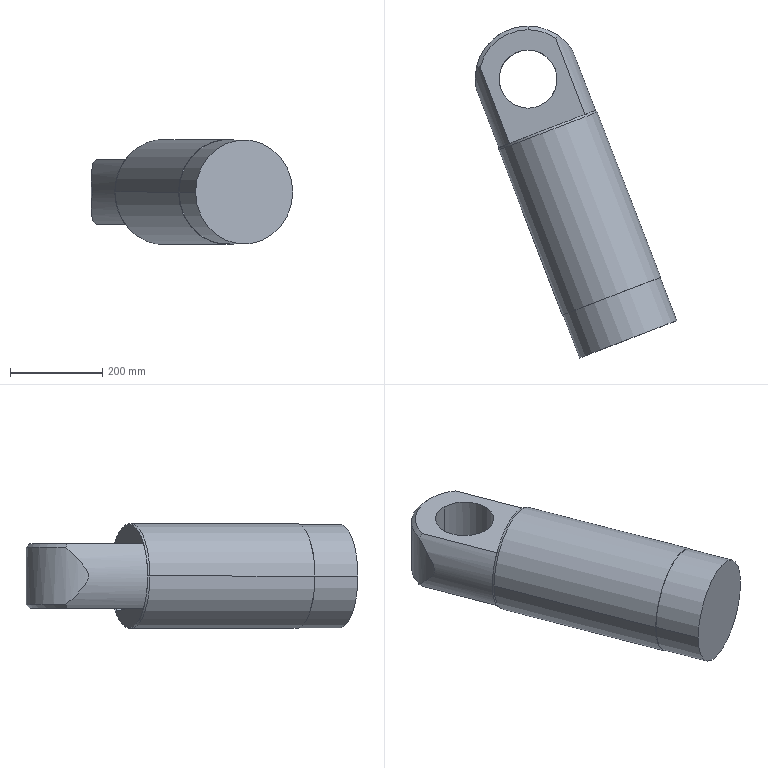Part | SolidWorks | features MoveFace 2, BaseBody 1, Scale 1 | 1 solid | 20 faces | box 436.641 x 719.533 x 228 mm | volume 24273606 mm3 | cylinder 10 | cone 5 | plane 5 | commonest cylinder face diameters 224.4 x3 228 x3 126 x2 225.6 x2
STEP:
#1=CARTESIAN_POINT('',(450.61,-136.711,89.501));
#2=VERTEX_POINT('',#1);
#3=CARTESIAN_POINT('',(237.813,-218.572,89.501));
#4=VERTEX_POINT('',#3);
#5=CARTESIAN_POINT('',(344.212,-177.641,89.501));
#6=DIRECTION('',(0.359,-0.9333,-0.000000526));
#7=DIRECTION('',(0.9333,0.359,0.));
#8=AXIS2_PLACEMENT_3D('',#5,#6,#7);
#9=CIRCLE('',#8,114.);
#10=EDGE_CURVE('',#2,#4,#9,.T.);
#11=ORIENTED_EDGE('',*,*,#10,.T.);
#12=CARTESIAN_POINT('',(375.469,-576.408,89.5));
#13=VERTEX_POINT('',#12);
#14=CARTESIAN_POINT('',(236.09,-214.092,89.501));
#15=DIRECTION('',(0.359,-0.9333,-0.000000526));
#16=VECTOR('',#15,1000.);
#17=LINE('',#14,#16);
#18=EDGE_CURVE('',#4,#13,#17,.T.);
#19=ORIENTED_EDGE('',*,*,#18,.T.);
#20=CARTESIAN_POINT('',(588.266,-494.547,89.5));
#21=VERTEX_POINT('',#20);
#22=CARTESIAN_POINT('',(481.867,-535.477,89.5));
#23=DIRECTION('',(-0.359,0.9333,0.000000526));
#24=DIRECTION('',(0.9333,0.359,0.));
#25=AXIS2_PLACEMENT_3D('',#22,#23,#24);
#26=CIRCLE('',#25,114.);
#27=EDGE_CURVE('',#13,#21,#26,.T.);
#28=ORIENTED_EDGE('',*,*,#27,.T.);
#29=CARTESIAN_POINT('',(448.887,-132.231,89.501));
#30=DIRECTION('',(0.359,-0.9333,-0.000000526));
#31=VECTOR('',#30,1000.);
#32=LINE('',#29,#31);
#33=EDGE_CURVE('',#2,#21,#32,.T.);
#34=ORIENTED_EDGE('',*,*,#33,.F.);
#35=EDGE_LOOP('',(#11,#19,#28,#34));
#36=FACE_OUTER_BOUND('',#35,.T.);
#37=CARTESIAN_POINT('',(342.488,-173.161,89.501));
#38=DIRECTION('',(0.359,-0.9333,-0.000000526));
#39=DIRECTION('',(0.9333,0.359,0.));
#40=AXIS2_PLACEMENT_3D('',#37,#38,#39);
#41=CYLINDRICAL_SURFACE('',#40,114.);
#42=ADVANCED_FACE('',(#36),#41,.T.);
#43=CARTESIAN_POINT('',(447.256,-132.858,89.501));
#44=VERTEX_POINT('',#43);
#45=CARTESIAN_POINT('',(237.72,-213.465,89.501));
#46=VERTEX_POINT('',#45);
#47=CARTESIAN_POINT('',(342.488,-173.161,89.501));
#48=DIRECTION('',(0.359,-0.9333,-0.000000526));
#49=DIRECTION('',(0.9333,0.359,0.));
#50=AXIS2_PLACEMENT_3D('',#47,#48,#49);
#51=CIRCLE('',#50,112.253);
#52=EDGE_CURVE('',#44,#46,#51,.T.);
#53=ORIENTED_EDGE('',*,*,#52,.T.);
#54=CARTESIAN_POINT('',(237.813,-218.572,89.501));
#55=DIRECTION('',(0.01817,-0.9998,-0.000000494));
#56=VECTOR('',#55,1000.);
#57=LINE('',#54,#56);
#58=EDGE_CURVE('',#46,#4,#57,.T.);
#59=ORIENTED_EDGE('',*,*,#58,.T.);
#60=ORIENTED_EDGE('',*,*,#10,.F.);
#61=CARTESIAN_POINT('',(450.61,-136.711,89.501));
#62=DIRECTION('',(0.6566,-0.7542,-0.000000494));
#63=VECTOR('',#62,1000.);
#64=LINE('',#61,#63);
#65=EDGE_CURVE('',#44,#2,#64,.T.);
#66=ORIENTED_EDGE('',*,*,#65,.F.);
#67=EDGE_LOOP('',(#53,#59,#60,#66));
#68=FACE_OUTER_BOUND('',#67,.T.);
#69=CARTESIAN_POINT('',(344.212,-177.641,89.501));
#70=DIRECTION('',(0.359,-0.9333,-0.000000526));
#71=DIRECTION('',(0.9333,0.359,0.));
#72=AXIS2_PLACEMENT_3D('',#69,#70,#71);
#73=CONICAL_SURFACE('',#72,114.,0.3491);
#74=ADVANCED_FACE('',(#68),#73,.T.);
#75=CARTESIAN_POINT('',(376.589,-575.977,89.5));
#76=VERTEX_POINT('',#75);
#77=CARTESIAN_POINT('',(587.146,-494.977,89.5));
#78=VERTEX_POINT('',#77);
#79=CARTESIAN_POINT('',(481.867,-535.477,89.5));
#80=DIRECTION('',(-0.359,0.9333,0.000000526));
#81=DIRECTION('',(0.9333,0.359,0.));
#82=AXIS2_PLACEMENT_3D('',#79,#80,#81);
#83=CIRCLE('',#82,112.8);
#84=EDGE_CURVE('',#76,#78,#83,.T.);
#85=ORIENTED_EDGE('',*,*,#84,.F.);
#86=CARTESIAN_POINT('',(412.564,-669.496,89.5));
#87=VERTEX_POINT('',#86);
#88=CARTESIAN_POINT('',(376.589,-575.977,89.5));
#89=DIRECTION('',(0.359,-0.9333,-0.000000526));
#90=VECTOR('',#89,1000.);
#91=LINE('',#88,#90);
#92=EDGE_CURVE('',#76,#87,#91,.T.);
#93=ORIENTED_EDGE('',*,*,#92,.T.);
#94=CARTESIAN_POINT('',(623.122,-588.496,89.5));
#95=VERTEX_POINT('',#94);
#96=CARTESIAN_POINT('',(517.843,-628.996,89.5));
#97=DIRECTION('',(-0.359,0.9333,0.000000526));
#98=DIRECTION('',(0.9333,0.359,0.));
#99=AXIS2_PLACEMENT_3D('',#96,#97,#98);
#100=CIRCLE('',#99,112.8);
#101=EDGE_CURVE('',#87,#95,#100,.T.);
#102=ORIENTED_EDGE('',*,*,#101,.T.);
#103=CARTESIAN_POINT('',(587.146,-494.977,89.5));
#104=DIRECTION('',(0.359,-0.9333,-0.000000526));
#105=VECTOR('',#104,1000.);
#106=LINE('',#103,#105);
#107=EDGE_CURVE('',#78,#95,#106,.T.);
#108=ORIENTED_EDGE('',*,*,#107,.F.);
#109=EDGE_LOOP('',(#85,#93,#102,#108));
#110=FACE_OUTER_BOUND('',#109,.T.);
#111=CARTESIAN_POINT('',(481.867,-535.477,89.5));
#112=DIRECTION('',(0.359,-0.9333,-0.000000526));
#113=DIRECTION('',(0.9333,0.359,0.));
#114=AXIS2_PLACEMENT_3D('',#111,#112,#113);
#115=CYLINDRICAL_SURFACE('',#114,112.8);
#116=ADVANCED_FACE('',(#110),#115,.T.);
#117=CARTESIAN_POINT('',(364.055,30.665,27.194));
#118=VERTEX_POINT('',#117);
#119=CARTESIAN_POINT('',(397.955,-4.846,89.501));
#120=VERTEX_POINT('',#119);
#121=CARTESIAN_POINT('',(364.055,30.665,27.194));
#122=CARTESIAN_POINT('',(368.33,27.792,31.626));
#123=CARTESIAN_POINT('',(372.271,24.726,36.163));
#124=CARTESIAN_POINT('',(377.725,19.913,43.145));
#125=CARTESIAN_POINT('',(379.466,18.274,45.502));
#126=CARTESIAN_POINT('',(382.796,14.941,50.287));
#127=CARTESIAN_POINT('',(384.384,13.247,52.716));
#128=CARTESIAN_POINT('',(387.401,9.835,57.667));
#129=CARTESIAN_POINT('',(388.829,8.115,60.189));
#130=CARTESIAN_POINT('',(390.836,5.557,64.084));
#131=CARTESIAN_POINT('',(391.482,4.709,65.401));
#132=CARTESIAN_POINT('',(392.723,3.034,68.085));
#133=CARTESIAN_POINT('',(393.317,2.207,69.453));
#134=CARTESIAN_POINT('',(394.433,0.6119,72.236));
#135=CARTESIAN_POINT('',(394.957,-0.1586,73.655));
#136=CARTESIAN_POINT('',(395.677,-1.243,75.843));
#137=CARTESIAN_POINT('',(395.907,-1.592,76.583));
#138=CARTESIAN_POINT('',(396.339,-2.259,78.089));
#139=CARTESIAN_POINT('',(396.543,-2.577,78.857));
#140=CARTESIAN_POINT('',(397.102,-3.458,81.187));
#141=CARTESIAN_POINT('',(397.408,-3.952,82.777));
#142=CARTESIAN_POINT('',(397.675,-4.387,84.835));
#143=CARTESIAN_POINT('',(397.723,-4.465,85.25));
#144=CARTESIAN_POINT('',(397.805,-4.6,86.088));
#145=CARTESIAN_POINT('',(397.841,-4.658,86.512));
#146=CARTESIAN_POINT('',(397.926,-4.798,87.788));
#147=CARTESIAN_POINT('',(397.955,-4.846,88.642));
#148=CARTESIAN_POINT('',(397.955,-4.846,89.501));
#149=B_SPLINE_CURVE_WITH_KNOTS('',3,(#121,#122,#123,#124,#125,#126,#127,#128,#129,#130,#131,#132,#133,#134,#135,#136,#137,#138,#139,#140,#141,#142,#143,#144,#145,#146,#147,#148),.UNSPECIFIED.,.F.,.F.,(4,2,2,2,2,2,2,2,2,2,2,2,2,4),(-0.08062,-0.06046,-0.05038,-0.04031,-0.03023,-0.02519,-0.02015,-0.01512,-0.0126,-0.01008,-0.005038,-0.003779,-0.002519,0.),.UNSPECIFIED.);
#150=EDGE_CURVE('',#118,#120,#149,.T.);
#151=ORIENTED_EDGE('',*,*,#150,.T.);
#152=CARTESIAN_POINT('',(447.207,-132.877,89.501));
#153=VERTEX_POINT('',#152);
#154=CARTESIAN_POINT('',(447.207,-132.877,89.501));
#155=DIRECTION('',(0.359,-0.9333,-0.000000526));
#156=VECTOR('',#155,1000.);
#157=LINE('',#154,#156);
#158=EDGE_CURVE('',#120,#153,#157,.T.);
#159=ORIENTED_EDGE('',*,*,#158,.T.);
#160=CARTESIAN_POINT('',(424.328,-141.679,19.501));
#161=VERTEX_POINT('',#160);
#162=CARTESIAN_POINT('',(342.488,-173.161,89.501));
#163=DIRECTION('',(0.359,-0.9333,-0.000000526));
#164=DIRECTION('',(0.9333,0.359,0.));
#165=AXIS2_PLACEMENT_3D('',#162,#163,#164);
#166=CIRCLE('',#165,112.2);
#167=EDGE_CURVE('',#161,#153,#166,.T.);
#168=ORIENTED_EDGE('',*,*,#167,.F.);
#169=CARTESIAN_POINT('',(360.734,23.632,19.501));
#170=VERTEX_POINT('',#169);
#171=CARTESIAN_POINT('',(424.328,-141.679,19.501));
#172=DIRECTION('',(-0.359,0.9333,0.000000526));
#173=VECTOR('',#172,1000.);
#174=LINE('',#171,#173);
#175=EDGE_CURVE('',#161,#170,#174,.T.);
#176=ORIENTED_EDGE('',*,*,#175,.T.);
#177=CARTESIAN_POINT('',(360.734,23.632,19.501));
#178=CARTESIAN_POINT('',(361.073,24.176,20.141));
#179=CARTESIAN_POINT('',(361.395,24.732,20.783));
#180=CARTESIAN_POINT('',(362.01,25.868,22.068));
#181=CARTESIAN_POINT('',(362.302,26.449,22.713));
#182=CARTESIAN_POINT('',(363.13,28.215,24.641));
#183=CARTESIAN_POINT('',(363.62,29.426,25.92));
#184=CARTESIAN_POINT('',(364.055,30.665,27.194));
#185=B_SPLINE_CURVE_WITH_KNOTS('',3,(#177,#178,#179,#180,#181,#182,#183,#184),.UNSPECIFIED.,.F.,.F.,(4,2,2,4),(0.01566,0.01836,0.02107,0.02648),.UNSPECIFIED.);
#186=EDGE_CURVE('',#170,#118,#185,.T.);
#187=ORIENTED_EDGE('',*,*,#186,.T.);
#188=EDGE_LOOP('',(#151,#159,#168,#176,#187));
#189=FACE_OUTER_BOUND('',#188,.T.);
#190=CARTESIAN_POINT('',(342.488,-173.161,89.501));
#191=DIRECTION('',(0.359,-0.9333,-0.000000526));
#192=DIRECTION('',(0.9333,0.359,0.));
#193=AXIS2_PLACEMENT_3D('',#190,#191,#192);
#194=CYLINDRICAL_SURFACE('',#193,112.2);
#195=ADVANCED_FACE('',(#189),#194,.T.);
#196=CARTESIAN_POINT('',(300.911,-128.083,19.501));
#197=VERTEX_POINT('',#196);
#198=CARTESIAN_POINT('',(300.911,-2.083,19.501));
#199=VERTEX_POINT('',#198);
#200=CARTESIAN_POINT('',(300.911,-128.083,19.501));
#201=CARTESIAN_POINT('',(296.788,-128.083,19.501));
#202=CARTESIAN_POINT('',(292.665,-127.677,19.501));
#203=CARTESIAN_POINT('',(284.577,-126.068,19.501));
#204=CARTESIAN_POINT('',(280.612,-124.865,19.501));
#205=CARTESIAN_POINT('',(272.993,-121.709,19.501));
#206=CARTESIAN_POINT('',(269.339,-119.756,19.501));
#207=CARTESIAN_POINT('',(262.482,-115.174,19.501));
#208=CARTESIAN_POINT('',(259.279,-112.546,19.501));
#209=CARTESIAN_POINT('',(253.448,-106.715,19.501));
#210=CARTESIAN_POINT('',(250.82,-103.512,19.501));
#211=CARTESIAN_POINT('',(246.238,-96.655,19.501));
#212=CARTESIAN_POINT('',(244.285,-93.001,19.501));
#213=CARTESIAN_POINT('',(241.129,-85.382,19.501));
#214=CARTESIAN_POINT('',(239.926,-81.417,19.501));
#215=CARTESIAN_POINT('',(238.318,-73.329,19.501));
#216=CARTESIAN_POINT('',(237.911,-69.206,19.501));
#217=CARTESIAN_POINT('',(237.911,-60.959,19.501));
#218=CARTESIAN_POINT('',(238.318,-56.836,19.501));
#219=CARTESIAN_POINT('',(239.926,-48.748,19.501));
#220=CARTESIAN_POINT('',(241.129,-44.783,19.501));
#221=CARTESIAN_POINT('',(244.285,-37.164,19.501));
#222=CARTESIAN_POINT('',(246.238,-33.51,19.501));
#223=CARTESIAN_POINT('',(250.82,-26.653,19.501));
#224=CARTESIAN_POINT('',(253.448,-23.451,19.501));
#225=CARTESIAN_POINT('',(259.279,-17.619,19.501));
#226=CARTESIAN_POINT('',(262.482,-14.991,19.501));
#227=CARTESIAN_POINT('',(269.339,-10.409,19.501));
#228=CARTESIAN_POINT('',(272.993,-8.456,19.501));
#229=CARTESIAN_POINT('',(280.612,-5.3,19.501));
#230=CARTESIAN_POINT('',(284.577,-4.098,19.501));
#231=CARTESIAN_POINT('',(292.665,-2.489,19.501));
#232=CARTESIAN_POINT('',(296.788,-2.083,19.501));
#233=CARTESIAN_POINT('',(300.911,-2.083,19.501));
#234=B_SPLINE_CURVE_WITH_KNOTS('',3,(#200,#201,#202,#203,#204,#205,#206,#207,#208,#209,#210,#211,#212,#213,#214,#215,#216,#217,#218,#219,#220,#221,#222,#223,#224,#225,#226,#227,#228,#229,#230,#231,#232,#233),.UNSPECIFIED.,.F.,.F.,(4,2,2,2,2,2,2,2,2,2,2,2,2,2,2,2,4),(0.,0.03125,0.0625,0.09375,0.125,0.1563,0.1875,0.2188,0.25,0.2813,0.3125,0.3438,0.375,0.4063,0.4375,0.4688,0.5),.UNSPECIFIED.);
#235=EDGE_CURVE('',#197,#199,#234,.T.);
#236=ORIENTED_EDGE('',*,*,#235,.T.);
#237=CARTESIAN_POINT('',(300.911,-2.083,159.501));
#238=VERTEX_POINT('',#237);
#239=CARTESIAN_POINT('',(300.911,-2.083,257.081));
#240=DIRECTION('',(-0.000000159,-0.000000625,1.));
#241=VECTOR('',#240,1000.);
#242=LINE('',#239,#241);
#243=EDGE_CURVE('',#199,#238,#242,.T.);
#244=ORIENTED_EDGE('',*,*,#243,.T.);
#245=CARTESIAN_POINT('',(300.911,-128.083,159.501));
#246=VERTEX_POINT('',#245);
#247=CARTESIAN_POINT('',(300.911,-2.083,159.501));
#248=CARTESIAN_POINT('',(296.788,-2.083,159.501));
#249=CARTESIAN_POINT('',(292.665,-2.489,159.501));
#250=CARTESIAN_POINT('',(284.577,-4.098,159.501));
#251=CARTESIAN_POINT('',(280.612,-5.3,159.501));
#252=CARTESIAN_POINT('',(272.993,-8.456,159.501));
#253=CARTESIAN_POINT('',(269.339,-10.409,159.501));
#254=CARTESIAN_POINT('',(262.482,-14.991,159.501));
#255=CARTESIAN_POINT('',(259.279,-17.619,159.501));
#256=CARTESIAN_POINT('',(253.448,-23.451,159.501));
#257=CARTESIAN_POINT('',(250.82,-26.653,159.501));
#258=CARTESIAN_POINT('',(246.238,-33.51,159.501));
#259=CARTESIAN_POINT('',(244.285,-37.164,159.501));
#260=CARTESIAN_POINT('',(241.129,-44.783,159.501));
#261=CARTESIAN_POINT('',(239.926,-48.748,159.501));
#262=CARTESIAN_POINT('',(238.318,-56.836,159.501));
#263=CARTESIAN_POINT('',(237.911,-60.959,159.501));
#264=CARTESIAN_POINT('',(237.911,-69.206,159.501));
#265=CARTESIAN_POINT('',(238.318,-73.329,159.501));
#266=CARTESIAN_POINT('',(239.926,-81.418,159.501));
#267=CARTESIAN_POINT('',(241.129,-85.382,159.501));
#268=CARTESIAN_POINT('',(244.285,-93.001,159.501));
#269=CARTESIAN_POINT('',(246.238,-96.655,159.501));
#270=CARTESIAN_POINT('',(250.82,-103.512,159.501));
#271=CARTESIAN_POINT('',(253.448,-106.715,159.501));
#272=CARTESIAN_POINT('',(259.279,-112.546,159.501));
#273=CARTESIAN_POINT('',(262.482,-115.174,159.501));
#274=CARTESIAN_POINT('',(269.339,-119.756,159.501));
#275=CARTESIAN_POINT('',(272.993,-121.709,159.501));
#276=CARTESIAN_POINT('',(280.612,-124.865,159.501));
#277=CARTESIAN_POINT('',(284.577,-126.068,159.501));
#278=CARTESIAN_POINT('',(292.665,-127.677,159.501));
#279=CARTESIAN_POINT('',(296.788,-128.083,159.501));
#280=CARTESIAN_POINT('',(300.911,-128.083,159.501));
#281=B_SPLINE_CURVE_WITH_KNOTS('',3,(#247,#248,#249,#250,#251,#252,#253,#254,#255,#256,#257,#258,#259,#260,#261,#262,#263,#264,#265,#266,#267,#268,#269,#270,#271,#272,#273,#274,#275,#276,#277,#278,#279,#280),.UNSPECIFIED.,.F.,.F.,(4,2,2,2,2,2,2,2,2,2,2,2,2,2,2,2,4),(0.5,0.5313,0.5625,0.5938,0.625,0.6563,0.6875,0.7188,0.75,0.7813,0.8125,0.8438,0.875,0.9063,0.9375,0.9688,1.),.UNSPECIFIED.);
#282=EDGE_CURVE('',#238,#246,#281,.T.);
#283=ORIENTED_EDGE('',*,*,#282,.T.);
#284=CARTESIAN_POINT('',(300.911,-128.083,257.081));
#285=DIRECTION('',(-0.000000159,-0.000000625,1.));
#286=VECTOR('',#285,1000.);
#287=LINE('',#284,#286);
#288=EDGE_CURVE('',#197,#246,#287,.T.);
#289=ORIENTED_EDGE('',*,*,#288,.F.);
#290=EDGE_LOOP('',(#236,#244,#283,#289));
#291=FACE_OUTER_BOUND('',#290,.T.);
#292=CARTESIAN_POINT('',(300.911,-65.083,257.081));
#293=DIRECTION('',(-0.000000159,-0.000000625,1.));
#294=DIRECTION('',(0.,-1.,-0.000000625));
#295=AXIS2_PLACEMENT_3D('',#292,#293,#294);
#296=CYLINDRICAL_SURFACE('',#295,63.);
#297=ADVANCED_FACE('',(#291),#296,.F.);
#298=CARTESIAN_POINT('',(197.056,-39.334,159.501));
#299=VERTEX_POINT('',#298);
#300=CARTESIAN_POINT('',(300.911,41.917,159.501));
#301=VERTEX_POINT('',#300);
#302=CARTESIAN_POINT('',(300.911,-65.083,159.501));
#303=DIRECTION('',(0.000000159,0.000000625,-1.));
#304=DIRECTION('',(0.,1.,0.000000625));
#305=AXIS2_PLACEMENT_3D('',#302,#303,#304);
#306=CIRCLE('',#305,107.);
#307=EDGE_CURVE('',#299,#301,#306,.T.);
#308=ORIENTED_EDGE('',*,*,#307,.T.);
#309=CARTESIAN_POINT('',(300.911,50.036,151.382));
#310=VERTEX_POINT('',#309);
#311=CARTESIAN_POINT('',(300.911,50.235,151.183));
#312=DIRECTION('',(0.000000113,0.7071,-0.7071));
#313=VECTOR('',#312,1000.);
#314=LINE('',#311,#313);
#315=EDGE_CURVE('',#301,#310,#314,.T.);
#316=ORIENTED_EDGE('',*,*,#315,.T.);
#317=CARTESIAN_POINT('',(189.878,-36.339,151.807));
#318=VERTEX_POINT('',#317);
#319=CARTESIAN_POINT('',(300.911,50.036,151.382));
#320=CARTESIAN_POINT('',(294.535,50.061,151.357));
#321=CARTESIAN_POINT('',(288.238,49.553,151.339));
#322=CARTESIAN_POINT('',(278.904,48.021,151.319));
#323=CARTESIAN_POINT('',(275.812,47.381,151.313));
#324=CARTESIAN_POINT('',(271.203,46.225,151.307));
#325=CARTESIAN_POINT('',(269.672,45.807,151.306));
#326=CARTESIAN_POINT('',(266.619,44.904,151.303));
#327=CARTESIAN_POINT('',(265.1,44.42,151.302));
#328=CARTESIAN_POINT('',(257.596,41.854,151.299));
#329=CARTESIAN_POINT('',(251.832,39.327,151.302));
#330=CARTESIAN_POINT('',(243.532,34.844,151.315));
#331=CARTESIAN_POINT('',(240.824,33.233,151.32));
#332=CARTESIAN_POINT('',(236.851,30.64,151.33));
#333=CARTESIAN_POINT('',(235.541,29.746,151.334));
#334=CARTESIAN_POINT('',(232.952,27.898,151.343));
#335=CARTESIAN_POINT('',(231.673,26.944,151.347));
#336=CARTESIAN_POINT('',(225.413,22.067,151.371));
#337=CARTESIAN_POINT('',(220.787,17.796,151.395));
#338=CARTESIAN_POINT('',(214.406,10.851,151.439));
#339=CARTESIAN_POINT('',(212.373,8.446,151.455));
#340=CARTESIAN_POINT('',(209.465,4.7,151.48));
#341=CARTESIAN_POINT('',(208.519,3.429,151.489));
#342=CARTESIAN_POINT('',(206.676,0.839,151.507));
#343=CARTESIAN_POINT('',(205.778,-0.4811,151.517));
#344=CARTESIAN_POINT('',(201.449,-7.137,151.566));
#345=CARTESIAN_POINT('',(198.473,-12.68,151.608));
#346=CARTESIAN_POINT('',(193.46,-24.188,151.702));
#347=CARTESIAN_POINT('',(191.423,-30.153,151.752));
#348=CARTESIAN_POINT('',(189.878,-36.339,151.807));
#349=B_SPLINE_CURVE_WITH_KNOTS('',3,(#319,#320,#321,#322,#323,#324,#325,#326,#327,#328,#329,#330,#331,#332,#333,#334,#335,#336,#337,#338,#339,#340,#341,#342,#343,#344,#345,#346,#347,#348),.UNSPECIFIED.,.F.,.F.,(4,2,2,2,2,2,2,2,2,2,2,2,2,2,4),(0.,0.01891,0.02837,0.0331,0.03783,0.05674,0.0662,0.07093,0.07565,0.09457,0.104,0.1088,0.1135,0.1324,0.1513),.UNSPECIFIED.);
#350=EDGE_CURVE('',#310,#318,#349,.T.);
#351=ORIENTED_EDGE('',*,*,#350,.T.);
#352=CARTESIAN_POINT('',(197.056,-39.334,159.501));
#353=CARTESIAN_POINT('',(196.44,-39.157,158.86));
#354=CARTESIAN_POINT('',(195.828,-38.96,158.218));
#355=CARTESIAN_POINT('',(194.61,-38.529,156.933));
#356=CARTESIAN_POINT('',(194.005,-38.294,156.288));
#357=CARTESIAN_POINT('',(192.206,-37.538,154.36));
#358=CARTESIAN_POINT('',(191.031,-36.968,153.081));
#359=CARTESIAN_POINT('',(189.878,-36.339,151.807));
#360=B_SPLINE_CURVE_WITH_KNOTS('',3,(#352,#353,#354,#355,#356,#357,#358,#359),.UNSPECIFIED.,.F.,.F.,(4,2,2,4),(0.01566,0.01836,0.02107,0.02648),.UNSPECIFIED.);
#361=EDGE_CURVE('',#299,#318,#360,.T.);
#362=ORIENTED_EDGE('',*,*,#361,.F.);
#363=EDGE_LOOP('',(#308,#316,#351,#362));
#364=FACE_OUTER_BOUND('',#363,.T.);
#365=CARTESIAN_POINT('',(300.911,-65.083,151.183));
#366=DIRECTION('',(0.000000159,0.000000625,-1.));
#367=DIRECTION('',(0.,1.,0.000000625));
#368=AXIS2_PLACEMENT_3D('',#365,#366,#367);
#369=CONICAL_SURFACE('',#368,115.317,0.7854);
#370=ADVANCED_FACE('',(#364),#369,.T.);
#371=ORIENTED_EDGE('',*,*,#18,.F.);
#372=CARTESIAN_POINT('',(344.212,-177.641,89.501));
#373=DIRECTION('',(0.359,-0.9333,-0.000000526));
#374=DIRECTION('',(0.9333,0.359,0.));
#375=AXIS2_PLACEMENT_3D('',#372,#373,#374);
#376=CIRCLE('',#375,114.);
#377=EDGE_CURVE('',#4,#2,#376,.T.);
#378=ORIENTED_EDGE('',*,*,#377,.T.);
#379=ORIENTED_EDGE('',*,*,#33,.T.);
#380=CARTESIAN_POINT('',(481.867,-535.477,89.5));
#381=DIRECTION('',(-0.359,0.9333,0.000000526));
#382=DIRECTION('',(0.9333,0.359,0.));
#383=AXIS2_PLACEMENT_3D('',#380,#381,#382);
#384=CIRCLE('',#383,114.);
#385=EDGE_CURVE('',#21,#13,#384,.T.);
#386=ORIENTED_EDGE('',*,*,#385,.T.);
#387=EDGE_LOOP('',(#371,#378,#379,#386));
#388=FACE_OUTER_BOUND('',#387,.T.);
#389=CARTESIAN_POINT('',(342.488,-173.161,89.501));
#390=DIRECTION('',(0.359,-0.9333,-0.000000526));
#391=DIRECTION('',(0.9333,0.359,0.));
#392=AXIS2_PLACEMENT_3D('',#389,#390,#391);
#393=CYLINDRICAL_SURFACE('',#392,114.);
#394=ADVANCED_FACE('',(#388),#393,.T.);
#395=CARTESIAN_POINT('',(481.867,-535.477,89.5));
#396=DIRECTION('',(-0.359,0.9333,0.000000526));
#397=DIRECTION('',(0.9333,0.359,0.));
#398=AXIS2_PLACEMENT_3D('',#395,#396,#397);
#399=CIRCLE('',#398,112.8);
#400=EDGE_CURVE('',#78,#76,#399,.T.);
#401=ORIENTED_EDGE('',*,*,#400,.T.);
#402=ORIENTED_EDGE('',*,*,#84,.T.);
#403=EDGE_LOOP('',(#401,#402));
#404=FACE_BOUND('',#403,.T.);
#405=ORIENTED_EDGE('',*,*,#385,.F.);
#406=ORIENTED_EDGE('',*,*,#27,.F.);
#407=EDGE_LOOP('',(#405,#406));
#408=FACE_OUTER_BOUND('',#407,.T.);
#409=CARTESIAN_POINT('',(481.867,-535.477,89.5));
#410=DIRECTION('',(0.359,-0.9333,-0.000000526));
#411=DIRECTION('',(0.9333,0.359,0.));
#412=AXIS2_PLACEMENT_3D('',#409,#410,#411);
#413=PLANE('',#412);
#414=ADVANCED_FACE('',(#404,#408),#413,.T.);
#415=ORIENTED_EDGE('',*,*,#58,.F.);
#416=CARTESIAN_POINT('',(342.488,-173.161,89.501));
#417=DIRECTION('',(0.359,-0.9333,-0.000000526));
#418=DIRECTION('',(0.9333,0.359,0.));
#419=AXIS2_PLACEMENT_3D('',#416,#417,#418);
#420=CIRCLE('',#419,112.253);
#421=EDGE_CURVE('',#46,#44,#420,.T.);
#422=ORIENTED_EDGE('',*,*,#421,.T.);
#423=ORIENTED_EDGE('',*,*,#65,.T.);
#424=ORIENTED_EDGE('',*,*,#377,.F.);
#425=EDGE_LOOP('',(#415,#422,#423,#424));
#426=FACE_OUTER_BOUND('',#425,.T.);
#427=CARTESIAN_POINT('',(344.212,-177.641,89.501));
#428=DIRECTION('',(0.359,-0.9333,-0.000000526));
#429=DIRECTION('',(0.9333,0.359,0.));
#430=AXIS2_PLACEMENT_3D('',#427,#428,#429);
#431=CONICAL_SURFACE('',#430,114.,0.3491);
#432=ADVANCED_FACE('',(#426),#431,.T.);
#433=ORIENTED_EDGE('',*,*,#92,.F.);
#434=ORIENTED_EDGE('',*,*,#400,.F.);
#435=ORIENTED_EDGE('',*,*,#107,.T.);
#436=CARTESIAN_POINT('',(517.843,-628.996,89.5));
#437=DIRECTION('',(-0.359,0.9333,0.000000526));
#438=DIRECTION('',(0.9333,0.359,0.));
#439=AXIS2_PLACEMENT_3D('',#436,#437,#438);
#440=CIRCLE('',#439,112.8);
#441=EDGE_CURVE('',#95,#87,#440,.T.);
#442=ORIENTED_EDGE('',*,*,#441,.T.);
#443=EDGE_LOOP('',(#433,#434,#435,#442));
#444=FACE_OUTER_BOUND('',#443,.T.);
#445=CARTESIAN_POINT('',(481.867,-535.477,89.5));
#446=DIRECTION('',(0.359,-0.9333,-0.000000526));
#447=DIRECTION('',(0.9333,0.359,0.));
#448=AXIS2_PLACEMENT_3D('',#445,#446,#447);
#449=CYLINDRICAL_SURFACE('',#448,112.8);
#450=ADVANCED_FACE('',(#444),#449,.T.);
#451=ORIENTED_EDGE('',*,*,#52,.F.);
#452=ORIENTED_EDGE('',*,*,#421,.F.);
#453=EDGE_LOOP('',(#451,#452));
#454=FACE_OUTER_BOUND('',#453,.T.);
#455=CARTESIAN_POINT('',(260.649,-204.644,159.501));
#456=VERTEX_POINT('',#455);
#457=CARTESIAN_POINT('',(260.649,-204.644,19.501));
#458=VERTEX_POINT('',#457);
#459=CARTESIAN_POINT('',(342.488,-173.161,89.501));
#460=DIRECTION('',(0.359,-0.9333,-0.000000526));
#461=DIRECTION('',(0.9333,0.359,0.));
#462=AXIS2_PLACEMENT_3D('',#459,#460,#461);
#463=CIRCLE('',#462,112.2);
#464=EDGE_CURVE('',#456,#458,#463,.T.);
#465=ORIENTED_EDGE('',*,*,#464,.T.);
#466=CARTESIAN_POINT('',(270.026,-201.037,19.501));
#467=DIRECTION('',(0.9333,0.359,0.000000373));
#468=VECTOR('',#467,1000.);
#469=LINE('',#466,#468);
#470=EDGE_CURVE('',#458,#161,#469,.T.);
#471=ORIENTED_EDGE('',*,*,#470,.T.);
#472=ORIENTED_EDGE('',*,*,#167,.T.);
#473=CARTESIAN_POINT('',(424.328,-141.679,159.501));
#474=VERTEX_POINT('',#473);
#475=CARTESIAN_POINT('',(342.488,-173.161,89.501));
#476=DIRECTION('',(0.359,-0.9333,-0.000000526));
#477=DIRECTION('',(0.9333,0.359,0.));
#478=AXIS2_PLACEMENT_3D('',#475,#476,#477);
#479=CIRCLE('',#478,112.2);
#480=EDGE_CURVE('',#153,#474,#479,.T.);
#481=ORIENTED_EDGE('',*,*,#480,.T.);
#482=CARTESIAN_POINT('',(414.951,-145.286,159.501));
#483=DIRECTION('',(-0.9333,-0.359,-0.000000373));
#484=VECTOR('',#483,1000.);
#485=LINE('',#482,#484);
#486=EDGE_CURVE('',#474,#456,#485,.T.);
#487=ORIENTED_EDGE('',*,*,#486,.T.);
#488=EDGE_LOOP('',(#465,#471,#472,#481,#487));
#489=FACE_BOUND('',#488,.T.);
#490=CARTESIAN_POINT('',(447.207,-132.877,89.501));
#491=DIRECTION('',(-0.359,0.9333,0.000000526));
#492=DIRECTION('',(-0.9333,-0.359,0.));
#493=AXIS2_PLACEMENT_3D('',#490,#491,#492);
#494=PLANE('',#493);
#495=ADVANCED_FACE('',(#454,#489),#494,.T.);
#496=ORIENTED_EDGE('',*,*,#441,.F.);
#497=ORIENTED_EDGE('',*,*,#101,.F.);
#498=EDGE_LOOP('',(#496,#497));
#499=FACE_OUTER_BOUND('',#498,.T.);
#500=CARTESIAN_POINT('',(629.842,-585.911,89.5));
#501=DIRECTION('',(0.359,-0.9333,-0.000000526));
#502=DIRECTION('',(0.9333,0.359,0.));
#503=AXIS2_PLACEMENT_3D('',#500,#501,#502);
#504=PLANE('',#503);
#505=ADVANCED_FACE('',(#499),#504,.T.);
#506=ORIENTED_EDGE('',*,*,#470,.F.);
#507=CARTESIAN_POINT('',(197.056,-39.334,19.501));
#508=VERTEX_POINT('',#507);
#509=CARTESIAN_POINT('',(197.056,-39.334,19.501));
#510=DIRECTION('',(0.359,-0.9333,-0.000000526));
#511=VECTOR('',#510,1000.);
#512=LINE('',#509,#511);
#513=EDGE_CURVE('',#508,#458,#512,.T.);
#514=ORIENTED_EDGE('',*,*,#513,.F.);
#515=CARTESIAN_POINT('',(300.911,-65.083,19.501));
#516=DIRECTION('',(-0.000000159,-0.000000625,1.));
#517=DIRECTION('',(0.,-1.,-0.000000625));
#518=AXIS2_PLACEMENT_3D('',#515,#516,#517);
#519=CIRCLE('',#518,107.);
#520=EDGE_CURVE('',#170,#508,#519,.T.);
#521=ORIENTED_EDGE('',*,*,#520,.F.);
#522=ORIENTED_EDGE('',*,*,#175,.F.);
#523=EDGE_LOOP('',(#506,#514,#521,#522));
#524=FACE_OUTER_BOUND('',#523,.T.);
#525=ORIENTED_EDGE('',*,*,#235,.F.);
#526=CARTESIAN_POINT('',(300.911,-2.083,19.501));
#527=CARTESIAN_POINT('',(305.035,-2.083,19.501));
#528=CARTESIAN_POINT('',(309.158,-2.489,19.501));
#529=CARTESIAN_POINT('',(317.246,-4.098,19.501));
#530=CARTESIAN_POINT('',(321.211,-5.3,19.501));
#531=CARTESIAN_POINT('',(328.83,-8.456,19.501));
#532=CARTESIAN_POINT('',(332.484,-10.409,19.501));
#533=CARTESIAN_POINT('',(339.341,-14.991,19.501));
#534=CARTESIAN_POINT('',(342.544,-17.619,19.501));
#535=CARTESIAN_POINT('',(348.375,-23.451,19.501));
#536=CARTESIAN_POINT('',(351.003,-26.653,19.501));
#537=CARTESIAN_POINT('',(355.585,-33.51,19.501));
#538=CARTESIAN_POINT('',(357.538,-37.164,19.501));
#539=CARTESIAN_POINT('',(360.694,-44.783,19.501));
#540=CARTESIAN_POINT('',(361.897,-48.748,19.501));
#541=CARTESIAN_POINT('',(363.505,-56.836,19.501));
#542=CARTESIAN_POINT('',(363.911,-60.959,19.501));
#543=CARTESIAN_POINT('',(363.911,-69.206,19.501));
#544=CARTESIAN_POINT('',(363.505,-73.329,19.501));
#545=CARTESIAN_POINT('',(361.897,-81.417,19.501));
#546=CARTESIAN_POINT('',(360.694,-85.382,19.501));
#547=CARTESIAN_POINT('',(357.538,-93.001,19.501));
#548=CARTESIAN_POINT('',(355.585,-96.655,19.501));
#549=CARTESIAN_POINT('',(351.003,-103.512,19.501));
#550=CARTESIAN_POINT('',(348.375,-106.715,19.501));
#551=CARTESIAN_POINT('',(342.544,-112.546,19.501));
#552=CARTESIAN_POINT('',(339.341,-115.174,19.501));
#553=CARTESIAN_POINT('',(332.484,-119.756,19.501));
#554=CARTESIAN_POINT('',(328.83,-121.709,19.501));
#555=CARTESIAN_POINT('',(321.211,-124.865,19.501));
#556=CARTESIAN_POINT('',(317.246,-126.068,19.501));
#557=CARTESIAN_POINT('',(309.158,-127.677,19.501));
#558=CARTESIAN_POINT('',(305.035,-128.083,19.501));
#559=CARTESIAN_POINT('',(300.911,-128.083,19.501));
#560=B_SPLINE_CURVE_WITH_KNOTS('',3,(#526,#527,#528,#529,#530,#531,#532,#533,#534,#535,#536,#537,#538,#539,#540,#541,#542,#543,#544,#545,#546,#547,#548,#549,#550,#551,#552,#553,#554,#555,#556,#557,#558,#559),.UNSPECIFIED.,.F.,.F.,(4,2,2,2,2,2,2,2,2,2,2,2,2,2,2,2,4),(0.5,0.5313,0.5625,0.5938,0.625,0.6563,0.6875,0.7188,0.75,0.7813,0.8125,0.8438,0.875,0.9063,0.9375,0.9688,1.),.UNSPECIFIED.);
#561=EDGE_CURVE('',#199,#197,#560,.T.);
#562=ORIENTED_EDGE('',*,*,#561,.F.);
#563=EDGE_LOOP('',(#525,#562));
#564=FACE_BOUND('',#563,.T.);
#565=CARTESIAN_POINT('',(498.894,-112.993,19.501));
#566=DIRECTION('',(-0.000000159,-0.000000625,1.));
#567=DIRECTION('',(0.,-1.,-0.000000625));
#568=AXIS2_PLACEMENT_3D('',#565,#566,#567);
#569=PLANE('',#568);
#570=ADVANCED_FACE('',(#524,#564),#569,.F.);
#571=CARTESIAN_POINT('',(260.649,-204.644,159.501));
#572=DIRECTION('',(-0.359,0.9333,0.000000526));
#573=VECTOR('',#572,1000.);
#574=LINE('',#571,#573);
#575=EDGE_CURVE('',#456,#299,#574,.T.);
#576=ORIENTED_EDGE('',*,*,#575,.T.);
#577=ORIENTED_EDGE('',*,*,#361,.T.);
#578=CARTESIAN_POINT('',(189.878,-36.339,27.194));
#579=VERTEX_POINT('',#578);
#580=CARTESIAN_POINT('',(189.878,-36.339,151.807));
#581=CARTESIAN_POINT('',(188.628,-41.344,147.369));
#582=CARTESIAN_POINT('',(187.758,-46.267,142.826));
#583=CARTESIAN_POINT('',(186.936,-53.503,135.835));
#584=CARTESIAN_POINT('',(186.742,-55.89,133.474));
#585=CARTESIAN_POINT('',(186.506,-60.601,128.681));
#586=CARTESIAN_POINT('',(186.463,-62.925,126.249));
#587=CARTESIAN_POINT('',(186.512,-67.485,121.29));
#588=CARTESIAN_POINT('',(186.605,-69.721,118.764));
#589=CARTESIAN_POINT('',(186.832,-72.967,114.863));
#590=CARTESIAN_POINT('',(186.921,-74.031,113.543));
#591=CARTESIAN_POINT('',(187.125,-76.107,110.853));
#592=CARTESIAN_POINT('',(187.238,-77.118,109.484));
#593=CARTESIAN_POINT('',(187.479,-79.05,106.694));
#594=CARTESIAN_POINT('',(187.607,-79.973,105.273));
#595=CARTESIAN_POINT('',(187.8,-81.259,103.079));
#596=CARTESIAN_POINT('',(187.864,-81.671,102.337));
#597=CARTESIAN_POINT('',(187.99,-82.454,100.827));
#598=CARTESIAN_POINT('',(188.051,-82.825,100.057));
#599=CARTESIAN_POINT('',(188.226,-83.848,97.723));
#600=CARTESIAN_POINT('',(188.33,-84.415,96.128));
#601=CARTESIAN_POINT('',(188.422,-84.91,94.062));
#602=CARTESIAN_POINT('',(188.438,-84.998,93.645));
#603=CARTESIAN_POINT('',(188.467,-85.15,92.803));
#604=CARTESIAN_POINT('',(188.479,-85.215,92.377));
#605=CARTESIAN_POINT('',(188.508,-85.368,91.105));
#606=CARTESIAN_POINT('',(188.518,-85.418,90.258));
#607=CARTESIAN_POINT('',(188.516,-85.41,88.565));
#608=CARTESIAN_POINT('',(188.505,-85.353,87.72));
#609=CARTESIAN_POINT('',(188.464,-85.135,86.03));
#610=CARTESIAN_POINT('',(188.433,-84.973,85.183));
#611=CARTESIAN_POINT('',(188.32,-84.362,82.705));
#612=CARTESIAN_POINT('',(188.215,-83.786,81.118));
#613=CARTESIAN_POINT('',(188.04,-82.756,78.798));
#614=CARTESIAN_POINT('',(187.978,-82.385,78.036));
#615=CARTESIAN_POINT('',(187.852,-81.597,76.528));
#616=CARTESIAN_POINT('',(187.788,-81.182,75.787));
#617=CARTESIAN_POINT('',(187.596,-79.893,73.601));
#618=CARTESIAN_POINT('',(187.469,-78.973,72.191));
#619=CARTESIAN_POINT('',(187.231,-77.055,69.431));
#620=CARTESIAN_POINT('',(187.119,-76.057,68.081));
#621=CARTESIAN_POINT('',(186.919,-74.004,65.424));
#622=CARTESIAN_POINT('',(186.83,-72.949,64.116));
#623=CARTESIAN_POINT('',(186.606,-69.723,60.24));
#624=CARTESIAN_POINT('',(186.512,-67.489,57.716));
#625=CARTESIAN_POINT('',(186.475,-64.06,53.986));
#626=CARTESIAN_POINT('',(186.48,-62.902,52.751));
#627=CARTESIAN_POINT('',(186.525,-60.572,50.307));
#628=CARTESIAN_POINT('',(186.566,-59.398,49.095));
#629=CARTESIAN_POINT('',(186.745,-55.855,45.491));
#630=CARTESIAN_POINT('',(186.939,-53.464,43.128));
#631=CARTESIAN_POINT('',(187.764,-46.227,36.137));
#632=CARTESIAN_POINT('',(188.635,-41.316,31.608));
#633=CARTESIAN_POINT('',(189.878,-36.339,27.194));
#634=B_SPLINE_CURVE_WITH_KNOTS('',3,(#580,#581,#582,#583,#584,#585,#586,#587,#588,#589,#590,#591,#592,#593,#594,#595,#596,#597,#598,#599,#600,#601,#602,#603,#604,#605,#606,#607,#608,#609,#610,#611,#612,#613,#614,#615,#616,#617,#618,#619,#620,#621,#622,#623,#624,#625,#626,#627,#628,#629,#630,#631,#632,#633),.UNSPECIFIED.,.F.,.F.,(4,2,2,2,2,2,2,2,2,2,2,2,2,2,2,2,2,2,2,2,2,2,2,2,2,2,4),(0.,0.02017,0.03026,0.04034,0.05043,0.05547,0.06051,0.06556,0.06808,0.0706,0.07564,0.0769,0.07816,0.08068,0.0832,0.08573,0.09077,0.09329,0.09581,0.1009,0.1059,0.1109,0.121,0.1261,0.1311,0.1412,0.1614),.UNSPECIFIED.);
#635=EDGE_CURVE('',#318,#579,#634,.T.);
#636=ORIENTED_EDGE('',*,*,#635,.T.);
#637=CARTESIAN_POINT('',(189.878,-36.339,27.194));
#638=CARTESIAN_POINT('',(192.196,-37.602,24.634));
#639=CARTESIAN_POINT('',(194.584,-38.623,22.071));
#640=CARTESIAN_POINT('',(197.056,-39.334,19.501));
#641=B_SPLINE_CURVE_WITH_KNOTS('',3,(#637,#638,#639,#640),.UNSPECIFIED.,.F.,.F.,(4,4),(0.,0.01091),.UNSPECIFIED.);
#642=EDGE_CURVE('',#579,#508,#641,.T.);
#643=ORIENTED_EDGE('',*,*,#642,.T.);
#644=ORIENTED_EDGE('',*,*,#513,.T.);
#645=ORIENTED_EDGE('',*,*,#464,.F.);
#646=EDGE_LOOP('',(#576,#577,#636,#643,#644,#645));
#647=FACE_OUTER_BOUND('',#646,.T.);
#648=CARTESIAN_POINT('',(342.488,-173.161,89.501));
#649=DIRECTION('',(0.359,-0.9333,-0.000000526));
#650=DIRECTION('',(0.9333,0.359,0.));
#651=AXIS2_PLACEMENT_3D('',#648,#649,#650);
#652=CYLINDRICAL_SURFACE('',#651,112.2);
#653=ADVANCED_FACE('',(#647),#652,.T.);
#654=ORIENTED_EDGE('',*,*,#486,.F.);
#655=CARTESIAN_POINT('',(360.734,23.632,159.501));
#656=VERTEX_POINT('',#655);
#657=CARTESIAN_POINT('',(360.734,23.632,159.501));
#658=DIRECTION('',(0.359,-0.9333,-0.000000526));
#659=VECTOR('',#658,1000.);
#660=LINE('',#657,#659);
#661=EDGE_CURVE('',#656,#474,#660,.T.);
#662=ORIENTED_EDGE('',*,*,#661,.F.);
#663=CARTESIAN_POINT('',(300.911,-65.083,159.501));
#664=DIRECTION('',(0.000000159,0.000000625,-1.));
#665=DIRECTION('',(0.,1.,0.000000625));
#666=AXIS2_PLACEMENT_3D('',#663,#664,#665);
#667=CIRCLE('',#666,107.);
#668=EDGE_CURVE('',#301,#656,#667,.T.);
#669=ORIENTED_EDGE('',*,*,#668,.F.);
#670=ORIENTED_EDGE('',*,*,#307,.F.);
#671=ORIENTED_EDGE('',*,*,#575,.F.);
#672=EDGE_LOOP('',(#654,#662,#669,#670,#671));
#673=FACE_OUTER_BOUND('',#672,.T.);
#674=CARTESIAN_POINT('',(300.911,-128.083,159.501));
#675=CARTESIAN_POINT('',(305.035,-128.083,159.501));
#676=CARTESIAN_POINT('',(309.158,-127.677,159.501));
#677=CARTESIAN_POINT('',(317.246,-126.068,159.501));
#678=CARTESIAN_POINT('',(321.211,-124.865,159.501));
#679=CARTESIAN_POINT('',(328.83,-121.709,159.501));
#680=CARTESIAN_POINT('',(332.484,-119.756,159.501));
#681=CARTESIAN_POINT('',(339.341,-115.174,159.501));
#682=CARTESIAN_POINT('',(342.544,-112.546,159.501));
#683=CARTESIAN_POINT('',(348.375,-106.715,159.501));
#684=CARTESIAN_POINT('',(351.003,-103.512,159.501));
#685=CARTESIAN_POINT('',(355.585,-96.655,159.501));
#686=CARTESIAN_POINT('',(357.538,-93.001,159.501));
#687=CARTESIAN_POINT('',(360.694,-85.382,159.501));
#688=CARTESIAN_POINT('',(361.897,-81.418,159.501));
#689=CARTESIAN_POINT('',(363.505,-73.329,159.501));
#690=CARTESIAN_POINT('',(363.911,-69.206,159.501));
#691=CARTESIAN_POINT('',(363.911,-60.959,159.501));
#692=CARTESIAN_POINT('',(363.505,-56.836,159.501));
#693=CARTESIAN_POINT('',(361.897,-48.748,159.501));
#694=CARTESIAN_POINT('',(360.694,-44.783,159.501));
#695=CARTESIAN_POINT('',(357.538,-37.164,159.501));
#696=CARTESIAN_POINT('',(355.585,-33.51,159.501));
#697=CARTESIAN_POINT('',(351.003,-26.653,159.501));
#698=CARTESIAN_POINT('',(348.375,-23.451,159.501));
#699=CARTESIAN_POINT('',(342.544,-17.619,159.501));
#700=CARTESIAN_POINT('',(339.341,-14.991,159.501));
#701=CARTESIAN_POINT('',(332.484,-10.409,159.501));
#702=CARTESIAN_POINT('',(328.83,-8.456,159.501));
#703=CARTESIAN_POINT('',(321.211,-5.3,159.501));
#704=CARTESIAN_POINT('',(317.246,-4.098,159.501));
#705=CARTESIAN_POINT('',(309.158,-2.489,159.501));
#706=CARTESIAN_POINT('',(305.035,-2.083,159.501));
#707=CARTESIAN_POINT('',(300.911,-2.083,159.501));
#708=B_SPLINE_CURVE_WITH_KNOTS('',3,(#674,#675,#676,#677,#678,#679,#680,#681,#682,#683,#684,#685,#686,#687,#688,#689,#690,#691,#692,#693,#694,#695,#696,#697,#698,#699,#700,#701,#702,#703,#704,#705,#706,#707),.UNSPECIFIED.,.F.,.F.,(4,2,2,2,2,2,2,2,2,2,2,2,2,2,2,2,4),(0.,0.03125,0.0625,0.09375,0.125,0.1563,0.1875,0.2188,0.25,0.2813,0.3125,0.3438,0.375,0.4063,0.4375,0.4688,0.5),.UNSPECIFIED.);
#709=EDGE_CURVE('',#246,#238,#708,.T.);
#710=ORIENTED_EDGE('',*,*,#709,.F.);
#711=ORIENTED_EDGE('',*,*,#282,.F.);
#712=EDGE_LOOP('',(#710,#711));
#713=FACE_BOUND('',#712,.T.);
#714=CARTESIAN_POINT('',(498.894,-112.994,159.501));
#715=DIRECTION('',(0.000000159,0.000000625,-1.));
#716=DIRECTION('',(0.,1.,0.000000625));
#717=AXIS2_PLACEMENT_3D('',#714,#715,#716);
#718=PLANE('',#717);
#719=ADVANCED_FACE('',(#673,#713),#718,.F.);
#720=ORIENTED_EDGE('',*,*,#158,.F.);
#721=CARTESIAN_POINT('',(364.055,30.665,151.807));
#722=VERTEX_POINT('',#721);
#723=CARTESIAN_POINT('',(397.955,-4.846,89.501));
#724=CARTESIAN_POINT('',(397.955,-4.846,91.229));
#725=CARTESIAN_POINT('',(397.837,-4.651,92.91));
#726=CARTESIAN_POINT('',(397.519,-4.133,95.373));
#727=CARTESIAN_POINT('',(397.389,-3.922,96.185));
#728=CARTESIAN_POINT('',(397.088,-3.439,97.793));
#729=CARTESIAN_POINT('',(396.916,-3.164,98.591));
#730=CARTESIAN_POINT('',(396.354,-2.28,100.93));
#731=CARTESIAN_POINT('',(395.919,-1.607,102.422));
#732=CARTESIAN_POINT('',(394.964,-0.1689,105.327));
#733=CARTESIAN_POINT('',(394.443,0.5973,106.738));
#734=CARTESIAN_POINT('',(393.334,2.183,109.508));
#735=CARTESIAN_POINT('',(392.745,3.003,110.866));
#736=CARTESIAN_POINT('',(391.509,4.673,113.544));
#737=CARTESIAN_POINT('',(390.862,5.524,114.867));
#738=CARTESIAN_POINT('',(388.85,8.089,118.774));
#739=CARTESIAN_POINT('',(387.419,9.814,121.304));
#740=CARTESIAN_POINT('',(384.397,13.234,126.267));
#741=CARTESIAN_POINT('',(382.806,14.931,128.699));
#742=CARTESIAN_POINT('',(379.472,18.269,133.492));
#743=CARTESIAN_POINT('',(377.728,19.91,135.852));
#744=CARTESIAN_POINT('',(372.27,24.727,142.84));
#745=CARTESIAN_POINT('',(368.328,27.793,147.377));
#746=CARTESIAN_POINT('',(364.055,30.665,151.807));
#747=B_SPLINE_CURVE_WITH_KNOTS('',3,(#723,#724,#725,#726,#727,#728,#729,#730,#731,#732,#733,#734,#735,#736,#737,#738,#739,#740,#741,#742,#743,#744,#745,#746),.UNSPECIFIED.,.F.,.F.,(4,2,2,2,2,2,2,2,2,2,2,4),(0.,0.005073,0.007609,0.01015,0.01522,0.02029,0.02536,0.03044,0.04058,0.05073,0.06087,0.08116),.UNSPECIFIED.);
#748=EDGE_CURVE('',#120,#722,#747,.T.);
#749=ORIENTED_EDGE('',*,*,#748,.T.);
#750=CARTESIAN_POINT('',(364.055,30.665,151.807));
#751=CARTESIAN_POINT('',(363.181,28.174,154.367));
#752=CARTESIAN_POINT('',(362.093,25.816,156.93));
#753=CARTESIAN_POINT('',(360.734,23.632,159.501));
#754=B_SPLINE_CURVE_WITH_KNOTS('',3,(#750,#751,#752,#753),.UNSPECIFIED.,.F.,.F.,(4,4),(0.,0.01091),.UNSPECIFIED.);
#755=EDGE_CURVE('',#722,#656,#754,.T.);
#756=ORIENTED_EDGE('',*,*,#755,.T.);
#757=ORIENTED_EDGE('',*,*,#661,.T.);
#758=ORIENTED_EDGE('',*,*,#480,.F.);
#759=EDGE_LOOP('',(#720,#749,#756,#757,#758));
#760=FACE_OUTER_BOUND('',#759,.T.);
#761=CARTESIAN_POINT('',(342.488,-173.161,89.501));
#762=DIRECTION('',(0.359,-0.9333,-0.000000526));
#763=DIRECTION('',(0.9333,0.359,0.));
#764=AXIS2_PLACEMENT_3D('',#761,#762,#763);
#765=CYLINDRICAL_SURFACE('',#764,112.2);
#766=ADVANCED_FACE('',(#760),#765,.T.);
#767=ORIENTED_EDGE('',*,*,#642,.F.);
#768=CARTESIAN_POINT('',(189.878,-36.339,27.194));
#769=CARTESIAN_POINT('',(190.991,-31.882,27.234));
#770=CARTESIAN_POINT('',(192.363,-27.532,27.271));
#771=CARTESIAN_POINT('',(195.606,-19.04,27.342));
#772=CARTESIAN_POINT('',(197.478,-14.899,27.375));
#773=CARTESIAN_POINT('',(200.665,-8.844,27.422));
#774=CARTESIAN_POINT('',(201.791,-6.852,27.437));
#775=CARTESIAN_POINT('',(204.172,-2.923,27.467));
#776=CARTESIAN_POINT('',(205.415,-1.005,27.481));
#777=CARTESIAN_POINT('',(209.301,4.616,27.521));
#778=CARTESIAN_POINT('',(212.099,8.184,27.545));
#779=CARTESIAN_POINT('',(218.101,14.969,27.589));
#780=CARTESIAN_POINT('',(221.306,18.185,27.608));
#781=CARTESIAN_POINT('',(225.573,21.98,27.629));
#782=CARTESIAN_POINT('',(226.44,22.728,27.633));
#783=CARTESIAN_POINT('',(228.2,24.201,27.641));
#784=CARTESIAN_POINT('',(229.092,24.925,27.644));
#785=CARTESIAN_POINT('',(231.79,27.047,27.655));
#786=CARTESIAN_POINT('',(233.623,28.402,27.661));
#787=CARTESIAN_POINT('',(239.226,32.29,27.678));
#788=CARTESIAN_POINT('',(243.096,34.645,27.686));
#789=CARTESIAN_POINT('',(251.104,38.889,27.698));
#790=CARTESIAN_POINT('',(255.243,40.778,27.701));
#791=CARTESIAN_POINT('',(260.589,42.836,27.701));
#792=CARTESIAN_POINT('',(261.668,43.233,27.7));
#793=CARTESIAN_POINT('',(263.831,43.991,27.7));
#794=CARTESIAN_POINT('',(264.915,44.353,27.699));
#795=CARTESIAN_POINT('',(268.178,45.389,27.697));
#796=CARTESIAN_POINT('',(270.365,46.011,27.695));
#797=CARTESIAN_POINT('',(276.966,47.678,27.687));
#798=CARTESIAN_POINT('',(281.415,48.523,27.678));
#799=CARTESIAN_POINT('',(288.164,49.393,27.661));
#800=CARTESIAN_POINT('',(290.426,49.616,27.655));
#801=CARTESIAN_POINT('',(293.837,49.849,27.645));
#802=CARTESIAN_POINT('',(294.978,49.91,27.641));
#803=CARTESIAN_POINT('',(297.265,49.998,27.633));
#804=CARTESIAN_POINT('',(298.413,50.024,27.629));
#805=CARTESIAN_POINT('',(304.149,50.071,27.608));
#806=CARTESIAN_POINT('',(308.696,49.831,27.589));
#807=CARTESIAN_POINT('',(317.705,48.82,27.545));
#808=CARTESIAN_POINT('',(322.169,48.047,27.521));
#809=CARTESIAN_POINT('',(328.802,46.487,27.481));
#810=CARTESIAN_POINT('',(331.002,45.899,27.467));
#811=CARTESIAN_POINT('',(335.382,44.588,27.438));
#812=CARTESIAN_POINT('',(337.566,43.861,27.422));
#813=CARTESIAN_POINT('',(344.014,41.497,27.375));
#814=CARTESIAN_POINT('',(348.191,39.674,27.342));
#815=CARTESIAN_POINT('',(356.304,35.538,27.271));
#816=CARTESIAN_POINT('',(360.241,33.227,27.234));
#817=CARTESIAN_POINT('',(364.055,30.665,27.194));
#818=B_SPLINE_CURVE_WITH_KNOTS('',3,(#768,#769,#770,#771,#772,#773,#774,#775,#776,#777,#778,#779,#780,#781,#782,#783,#784,#785,#786,#787,#788,#789,#790,#791,#792,#793,#794,#795,#796,#797,#798,#799,#800,#801,#802,#803,#804,#805,#806,#807,#808,#809,#810,#811,#812,#813,#814,#815,#816,#817),.UNSPECIFIED.,.F.,.F.,(4,2,2,2,2,2,2,2,2,2,2,2,2,2,2,2,2,2,2,2,2,2,2,2,4),(0.,0.01363,0.02726,0.03407,0.04089,0.05452,0.06815,0.07155,0.07496,0.08178,0.09541,0.109,0.1124,0.1158,0.1227,0.1363,0.1431,0.1465,0.1499,0.1636,0.1772,0.184,0.1908,0.2044,0.2181),.UNSPECIFIED.);
#819=EDGE_CURVE('',#579,#118,#818,.T.);
#820=ORIENTED_EDGE('',*,*,#819,.T.);
#821=ORIENTED_EDGE('',*,*,#186,.F.);
#822=ORIENTED_EDGE('',*,*,#520,.T.);
#823=EDGE_LOOP('',(#767,#820,#821,#822));
#824=FACE_OUTER_BOUND('',#823,.T.);
#825=CARTESIAN_POINT('',(300.911,-65.083,27.816));
#826=DIRECTION('',(-0.000000159,-0.000000625,1.));
#827=DIRECTION('',(0.,-1.,-0.000000625));
#828=AXIS2_PLACEMENT_3D('',#825,#826,#827);
#829=CONICAL_SURFACE('',#828,115.315,0.7854);
#830=ADVANCED_FACE('',(#824),#829,.T.);
#831=ORIENTED_EDGE('',*,*,#243,.F.);
#832=ORIENTED_EDGE('',*,*,#561,.T.);
#833=ORIENTED_EDGE('',*,*,#288,.T.);
#834=ORIENTED_EDGE('',*,*,#709,.T.);
#835=EDGE_LOOP('',(#831,#832,#833,#834));
#836=FACE_OUTER_BOUND('',#835,.T.);
#837=CARTESIAN_POINT('',(300.911,-65.083,257.081));
#838=DIRECTION('',(-0.000000159,-0.000000625,1.));
#839=DIRECTION('',(0.,-1.,-0.000000625));
#840=AXIS2_PLACEMENT_3D('',#837,#838,#839);
#841=CYLINDRICAL_SURFACE('',#840,63.);
#842=ADVANCED_FACE('',(#836),#841,.F.);
#843=ORIENTED_EDGE('',*,*,#315,.F.);
#844=ORIENTED_EDGE('',*,*,#668,.T.);
#845=ORIENTED_EDGE('',*,*,#755,.F.);
#846=CARTESIAN_POINT('',(364.055,30.665,151.807));
#847=CARTESIAN_POINT('',(359.386,33.801,151.759));
#848=CARTESIAN_POINT('',(354.538,36.56,151.714));
#849=CARTESIAN_POINT('',(344.496,41.344,151.629));
#850=CARTESIAN_POINT('',(339.302,43.371,151.59));
#851=CARTESIAN_POINT('',(332.586,45.432,151.545));
#852=CARTESIAN_POINT('',(331.235,45.819,151.536));
#853=CARTESIAN_POINT('',(328.529,46.542,151.519));
#854=CARTESIAN_POINT('',(327.172,46.877,151.511));
#855=CARTESIAN_POINT('',(323.09,47.808,151.486));
#856=CARTESIAN_POINT('',(320.354,48.326,151.471));
#857=CARTESIAN_POINT('',(312.099,49.58,151.428));
#858=CARTESIAN_POINT('',(306.536,50.015,151.403));
#859=CARTESIAN_POINT('',(300.911,50.036,151.382));
#860=B_SPLINE_CURVE_WITH_KNOTS('',3,(#846,#847,#848,#849,#850,#851,#852,#853,#854,#855,#856,#857,#858,#859),.UNSPECIFIED.,.F.,.F.,(4,2,2,2,2,2,4),(-0.06674,-0.05005,-0.03337,-0.0292,-0.02503,-0.01668,0.),.UNSPECIFIED.);
#861=EDGE_CURVE('',#722,#310,#860,.T.);
#862=ORIENTED_EDGE('',*,*,#861,.T.);
#863=EDGE_LOOP('',(#843,#844,#845,#862));
#864=FACE_OUTER_BOUND('',#863,.T.);
#865=CARTESIAN_POINT('',(300.911,-65.083,151.183));
#866=DIRECTION('',(0.000000159,0.000000625,-1.));
#867=DIRECTION('',(0.,1.,0.000000625));
#868=AXIS2_PLACEMENT_3D('',#865,#866,#867);
#869=CONICAL_SURFACE('',#868,115.317,0.7854);
#870=ADVANCED_FACE('',(#864),#869,.T.);
#871=ORIENTED_EDGE('',*,*,#150,.F.);
#872=ORIENTED_EDGE('',*,*,#819,.F.);
#873=ORIENTED_EDGE('',*,*,#635,.F.);
#874=ORIENTED_EDGE('',*,*,#350,.F.);
#875=ORIENTED_EDGE('',*,*,#861,.F.);
#876=ORIENTED_EDGE('',*,*,#748,.F.);
#877=EDGE_LOOP('',(#871,#872,#873,#874,#875,#876));
#878=FACE_OUTER_BOUND('',#877,.T.);
#879=CARTESIAN_POINT('',(300.481,-63.963,257.081));
#880=DIRECTION('',(-0.000000159,-0.000000625,1.));
#881=DIRECTION('',(0.,-1.,-0.000000625));
#882=AXIS2_PLACEMENT_3D('',#879,#880,#881);
#883=CYLINDRICAL_SURFACE('',#882,114.);
#884=ADVANCED_FACE('',(#878),#883,.T.);
#885=CLOSED_SHELL('',(#42,#74,#116,#195,#297,#370,#394,#414,#432,#450,#495,#505,#570,#653,#719,#766,#830,#842,#870,#884));
#886=MANIFOLD_SOLID_BREP('',#885);
#887=CARTESIAN_POINT('',(0.,0.,0.));
#888=DIRECTION('',(0.,0.,1.));
#889=DIRECTION('',(1.,0.,0.));
#890=AXIS2_PLACEMENT_3D('',#887,#888,#889);
#891=(LENGTH_UNIT()NAMED_UNIT(*)SI_UNIT(.MILLI.,.METRE.));
#892=UNCERTAINTY_MEASURE_WITH_UNIT(LENGTH_MEASURE(0.00001),#891,'','');
#893=(NAMED_UNIT(*)PLANE_ANGLE_UNIT()SI_UNIT($,.RADIAN.));
#894=(NAMED_UNIT(*)SI_UNIT($,.STERADIAN.)SOLID_ANGLE_UNIT());
#895=(GEOMETRIC_REPRESENTATION_CONTEXT(3)GLOBAL_UNCERTAINTY_ASSIGNED_CONTEXT((#892))GLOBAL_UNIT_ASSIGNED_CONTEXT((#891,#893,#894))REPRESENTATION_CONTEXT('',''));
#896=ADVANCED_BREP_SHAPE_REPRESENTATION('',(#886,#890),#895);